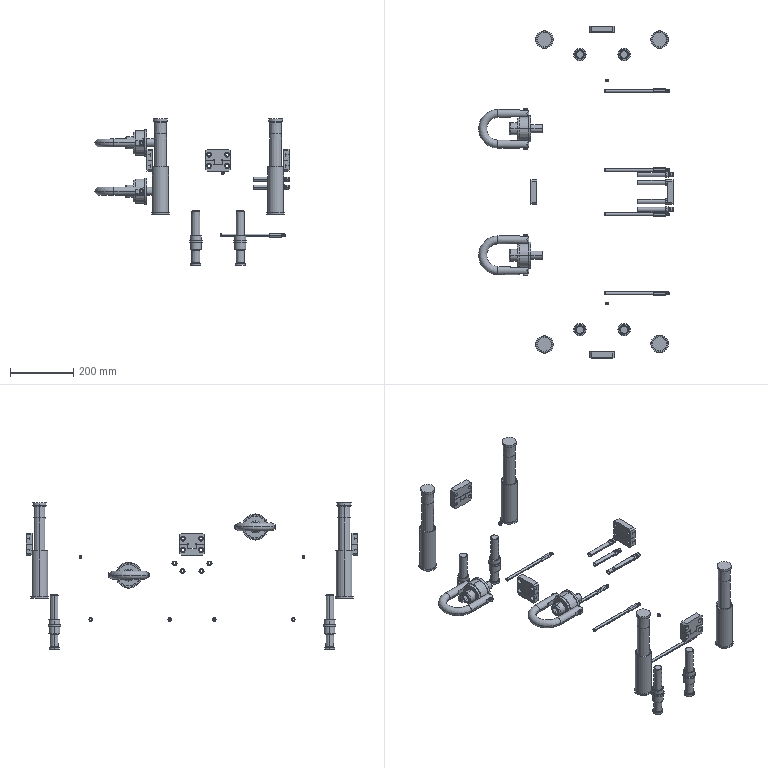Part | STEP file | 1 | 36 solids | 1266 faces | box 615.081 x 1049 x 462.275 mm | volume 3467998 mm3 | cylinder 568 | plane 438 | cone 252 | torus 8 | commonest cylinder face diameters 10.312 x48 15.875 x48 3.048 x40 38.113 x36 12.832 x32 16.497 x32